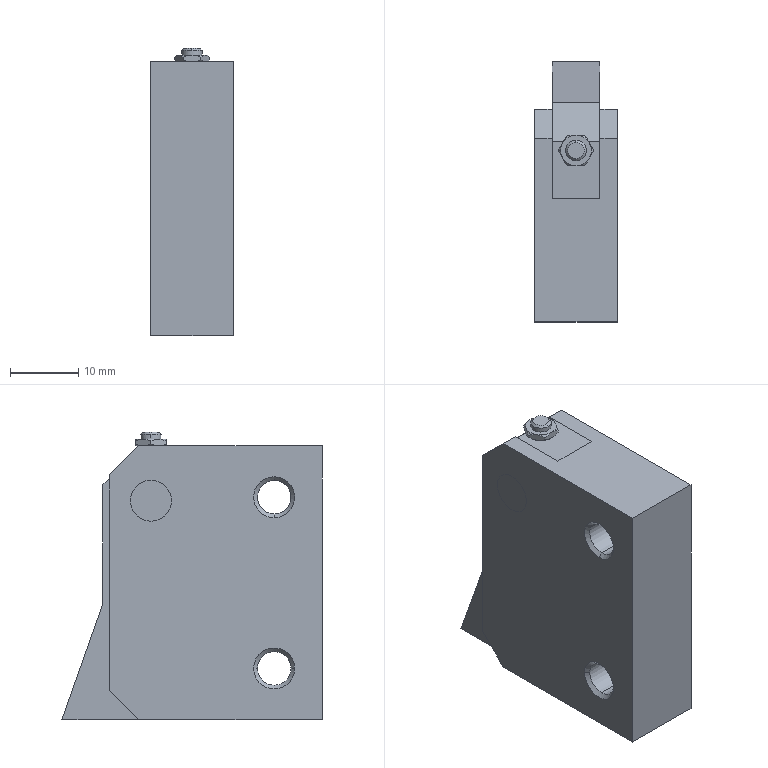Part | STEP file | Stopper Assembly PFC01-7SA-R-MK | 2 solids | 88 faces | box 12 x 38 x 42 mm | volume 13788 mm3 | plane 39 | cone 28 | cylinder 21 | commonest cylinder face diameters 6 x10 4.917 x6 3 x3 2.459 x2